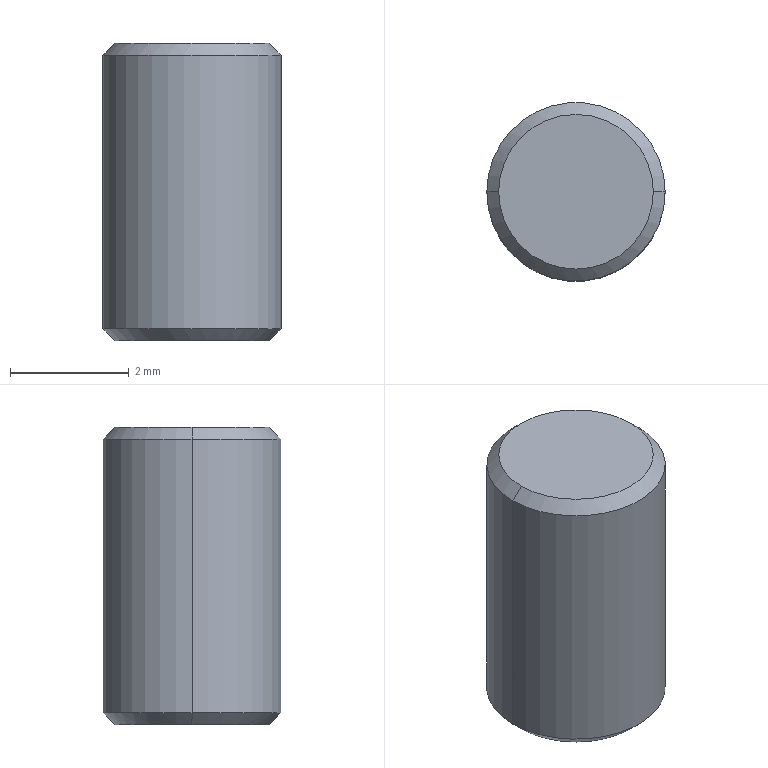Part | SolidWorks | features Chamfer 1, Extrusion 1 | 1 solid | 8 faces | box 3 x 3 x 5 mm | volume 34.983 mm3 | cone 4 | cylinder 2 | plane 2 | commonest cylinder face diameters 3 x2
STEP:
#1=CARTESIAN_POINT('',(1.3,0.,5.));
#2=VERTEX_POINT('',#1);
#3=CARTESIAN_POINT('',(-1.3,0.,5.));
#4=VERTEX_POINT('',#3);
#5=CARTESIAN_POINT('',(0.,0.,5.));
#6=DIRECTION('',(0.,0.,1.));
#7=DIRECTION('',(1.,0.,0.));
#8=AXIS2_PLACEMENT_3D('',#5,#6,#7);
#9=CIRCLE('',#8,1.3);
#10=EDGE_CURVE('',#2,#4,#9,.T.);
#11=ORIENTED_EDGE('',*,*,#10,.F.);
#12=CARTESIAN_POINT('',(1.5,0.,4.8));
#13=VERTEX_POINT('',#12);
#14=CARTESIAN_POINT('',(1.3,0.,5.));
#15=DIRECTION('',(0.7071,0.,-0.7071));
#16=VECTOR('',#15,1000.);
#17=LINE('',#14,#16);
#18=EDGE_CURVE('',#2,#13,#17,.T.);
#19=ORIENTED_EDGE('',*,*,#18,.T.);
#20=CARTESIAN_POINT('',(-1.5,0.,4.8));
#21=VERTEX_POINT('',#20);
#22=CARTESIAN_POINT('',(0.,0.,4.8));
#23=DIRECTION('',(0.,0.,-1.));
#24=DIRECTION('',(1.,0.,0.));
#25=AXIS2_PLACEMENT_3D('',#22,#23,#24);
#26=CIRCLE('',#25,1.5);
#27=EDGE_CURVE('',#21,#13,#26,.T.);
#28=ORIENTED_EDGE('',*,*,#27,.F.);
#29=CARTESIAN_POINT('',(-1.3,0.,5.));
#30=DIRECTION('',(-0.7071,0.,-0.7071));
#31=VECTOR('',#30,1000.);
#32=LINE('',#29,#31);
#33=EDGE_CURVE('',#4,#21,#32,.T.);
#34=ORIENTED_EDGE('',*,*,#33,.F.);
#35=EDGE_LOOP('',(#11,#19,#28,#34));
#36=FACE_OUTER_BOUND('',#35,.T.);
#37=CARTESIAN_POINT('',(0.,0.,5.));
#38=DIRECTION('',(0.,0.,-1.));
#39=DIRECTION('',(-1.,0.,0.));
#40=AXIS2_PLACEMENT_3D('',#37,#38,#39);
#41=CONICAL_SURFACE('',#40,1.3,0.7854);
#42=ADVANCED_FACE('',(#36),#41,.T.);
#43=CARTESIAN_POINT('',(-1.3,0.,0.));
#44=VERTEX_POINT('',#43);
#45=CARTESIAN_POINT('',(1.3,0.,0.));
#46=VERTEX_POINT('',#45);
#47=CARTESIAN_POINT('',(0.,0.,0.));
#48=DIRECTION('',(0.,0.,-1.));
#49=DIRECTION('',(1.,0.,0.));
#50=AXIS2_PLACEMENT_3D('',#47,#48,#49);
#51=CIRCLE('',#50,1.3);
#52=EDGE_CURVE('',#44,#46,#51,.T.);
#53=ORIENTED_EDGE('',*,*,#52,.F.);
#54=CARTESIAN_POINT('',(-1.5,0.,0.2));
#55=VERTEX_POINT('',#54);
#56=CARTESIAN_POINT('',(-1.5,0.,0.2));
#57=DIRECTION('',(-0.7071,0.,0.7071));
#58=VECTOR('',#57,1000.);
#59=LINE('',#56,#58);
#60=EDGE_CURVE('',#44,#55,#59,.T.);
#61=ORIENTED_EDGE('',*,*,#60,.T.);
#62=CARTESIAN_POINT('',(1.5,0.,0.2));
#63=VERTEX_POINT('',#62);
#64=CARTESIAN_POINT('',(0.,0.,0.2));
#65=DIRECTION('',(0.,0.,1.));
#66=DIRECTION('',(1.,0.,0.));
#67=AXIS2_PLACEMENT_3D('',#64,#65,#66);
#68=CIRCLE('',#67,1.5);
#69=EDGE_CURVE('',#63,#55,#68,.T.);
#70=ORIENTED_EDGE('',*,*,#69,.F.);
#71=CARTESIAN_POINT('',(1.5,0.,0.2));
#72=DIRECTION('',(0.7071,0.,0.7071));
#73=VECTOR('',#72,1000.);
#74=LINE('',#71,#73);
#75=EDGE_CURVE('',#46,#63,#74,.T.);
#76=ORIENTED_EDGE('',*,*,#75,.F.);
#77=EDGE_LOOP('',(#53,#61,#70,#76));
#78=FACE_OUTER_BOUND('',#77,.T.);
#79=CARTESIAN_POINT('',(0.,0.,0.2));
#80=DIRECTION('',(0.,0.,1.));
#81=DIRECTION('',(1.,0.,0.));
#82=AXIS2_PLACEMENT_3D('',#79,#80,#81);
#83=CONICAL_SURFACE('',#82,1.5,0.7854);
#84=ADVANCED_FACE('',(#78),#83,.T.);
#85=ORIENTED_EDGE('',*,*,#27,.T.);
#86=CARTESIAN_POINT('',(1.5,0.,5.));
#87=DIRECTION('',(0.,0.,-1.));
#88=VECTOR('',#87,1000.);
#89=LINE('',#86,#88);
#90=EDGE_CURVE('',#13,#63,#89,.T.);
#91=ORIENTED_EDGE('',*,*,#90,.T.);
#92=ORIENTED_EDGE('',*,*,#69,.T.);
#93=CARTESIAN_POINT('',(-1.5,0.,5.));
#94=DIRECTION('',(0.,0.,-1.));
#95=VECTOR('',#94,1000.);
#96=LINE('',#93,#95);
#97=EDGE_CURVE('',#21,#55,#96,.T.);
#98=ORIENTED_EDGE('',*,*,#97,.F.);
#99=EDGE_LOOP('',(#85,#91,#92,#98));
#100=FACE_OUTER_BOUND('',#99,.T.);
#101=CARTESIAN_POINT('',(0.,0.,5.));
#102=DIRECTION('',(0.,0.,-1.));
#103=DIRECTION('',(-1.,0.,0.));
#104=AXIS2_PLACEMENT_3D('',#101,#102,#103);
#105=CYLINDRICAL_SURFACE('',#104,1.5);
#106=ADVANCED_FACE('',(#100),#105,.T.);
#107=ORIENTED_EDGE('',*,*,#90,.F.);
#108=CARTESIAN_POINT('',(0.,0.,4.8));
#109=DIRECTION('',(0.,0.,-1.));
#110=DIRECTION('',(1.,0.,0.));
#111=AXIS2_PLACEMENT_3D('',#108,#109,#110);
#112=CIRCLE('',#111,1.5);
#113=EDGE_CURVE('',#13,#21,#112,.T.);
#114=ORIENTED_EDGE('',*,*,#113,.T.);
#115=ORIENTED_EDGE('',*,*,#97,.T.);
#116=CARTESIAN_POINT('',(0.,0.,0.2));
#117=DIRECTION('',(0.,0.,1.));
#118=DIRECTION('',(1.,0.,0.));
#119=AXIS2_PLACEMENT_3D('',#116,#117,#118);
#120=CIRCLE('',#119,1.5);
#121=EDGE_CURVE('',#55,#63,#120,.T.);
#122=ORIENTED_EDGE('',*,*,#121,.T.);
#123=EDGE_LOOP('',(#107,#114,#115,#122));
#124=FACE_OUTER_BOUND('',#123,.T.);
#125=CARTESIAN_POINT('',(0.,0.,5.));
#126=DIRECTION('',(0.,0.,-1.));
#127=DIRECTION('',(-1.,0.,0.));
#128=AXIS2_PLACEMENT_3D('',#125,#126,#127);
#129=CYLINDRICAL_SURFACE('',#128,1.5);
#130=ADVANCED_FACE('',(#124),#129,.T.);
#131=CARTESIAN_POINT('',(0.,0.,5.));
#132=DIRECTION('',(0.,0.,1.));
#133=DIRECTION('',(1.,0.,0.));
#134=AXIS2_PLACEMENT_3D('',#131,#132,#133);
#135=CIRCLE('',#134,1.3);
#136=EDGE_CURVE('',#4,#2,#135,.T.);
#137=ORIENTED_EDGE('',*,*,#136,.T.);
#138=ORIENTED_EDGE('',*,*,#10,.T.);
#139=EDGE_LOOP('',(#137,#138));
#140=FACE_OUTER_BOUND('',#139,.T.);
#141=CARTESIAN_POINT('',(0.,0.,5.));
#142=DIRECTION('',(0.,0.,1.));
#143=DIRECTION('',(1.,0.,0.));
#144=AXIS2_PLACEMENT_3D('',#141,#142,#143);
#145=PLANE('',#144);
#146=ADVANCED_FACE('',(#140),#145,.T.);
#147=CARTESIAN_POINT('',(0.,0.,0.));
#148=DIRECTION('',(0.,0.,-1.));
#149=DIRECTION('',(1.,0.,0.));
#150=AXIS2_PLACEMENT_3D('',#147,#148,#149);
#151=CIRCLE('',#150,1.3);
#152=EDGE_CURVE('',#46,#44,#151,.T.);
#153=ORIENTED_EDGE('',*,*,#152,.T.);
#154=ORIENTED_EDGE('',*,*,#52,.T.);
#155=EDGE_LOOP('',(#153,#154));
#156=FACE_OUTER_BOUND('',#155,.T.);
#157=CARTESIAN_POINT('',(0.,0.,0.));
#158=DIRECTION('',(0.,0.,1.));
#159=DIRECTION('',(1.,0.,0.));
#160=AXIS2_PLACEMENT_3D('',#157,#158,#159);
#161=PLANE('',#160);
#162=ADVANCED_FACE('',(#156),#161,.F.);
#163=ORIENTED_EDGE('',*,*,#60,.F.);
#164=ORIENTED_EDGE('',*,*,#152,.F.);
#165=ORIENTED_EDGE('',*,*,#75,.T.);
#166=ORIENTED_EDGE('',*,*,#121,.F.);
#167=EDGE_LOOP('',(#163,#164,#165,#166));
#168=FACE_OUTER_BOUND('',#167,.T.);
#169=CARTESIAN_POINT('',(0.,0.,0.2));
#170=DIRECTION('',(0.,0.,1.));
#171=DIRECTION('',(1.,0.,0.));
#172=AXIS2_PLACEMENT_3D('',#169,#170,#171);
#173=CONICAL_SURFACE('',#172,1.5,0.7854);
#174=ADVANCED_FACE('',(#168),#173,.T.);
#175=ORIENTED_EDGE('',*,*,#18,.F.);
#176=ORIENTED_EDGE('',*,*,#136,.F.);
#177=ORIENTED_EDGE('',*,*,#33,.T.);
#178=ORIENTED_EDGE('',*,*,#113,.F.);
#179=EDGE_LOOP('',(#175,#176,#177,#178));
#180=FACE_OUTER_BOUND('',#179,.T.);
#181=CARTESIAN_POINT('',(0.,0.,5.));
#182=DIRECTION('',(0.,0.,-1.));
#183=DIRECTION('',(-1.,0.,0.));
#184=AXIS2_PLACEMENT_3D('',#181,#182,#183);
#185=CONICAL_SURFACE('',#184,1.3,0.7854);
#186=ADVANCED_FACE('',(#180),#185,.T.);
#187=CLOSED_SHELL('',(#42,#84,#106,#130,#146,#162,#174,#186));
#188=MANIFOLD_SOLID_BREP('',#187);
#189=CARTESIAN_POINT('',(0.,0.,0.));
#190=DIRECTION('',(0.,0.,1.));
#191=DIRECTION('',(1.,0.,0.));
#192=AXIS2_PLACEMENT_3D('',#189,#190,#191);
#193=(LENGTH_UNIT()NAMED_UNIT(*)SI_UNIT(.MILLI.,.METRE.));
#194=UNCERTAINTY_MEASURE_WITH_UNIT(LENGTH_MEASURE(0.00001),#193,'','');
#195=(NAMED_UNIT(*)PLANE_ANGLE_UNIT()SI_UNIT($,.RADIAN.));
#196=(NAMED_UNIT(*)SI_UNIT($,.STERADIAN.)SOLID_ANGLE_UNIT());
#197=(GEOMETRIC_REPRESENTATION_CONTEXT(3)GLOBAL_UNCERTAINTY_ASSIGNED_CONTEXT((#194))GLOBAL_UNIT_ASSIGNED_CONTEXT((#193,#195,#196))REPRESENTATION_CONTEXT('',''));
#198=ADVANCED_BREP_SHAPE_REPRESENTATION('',(#188,#192),#197);